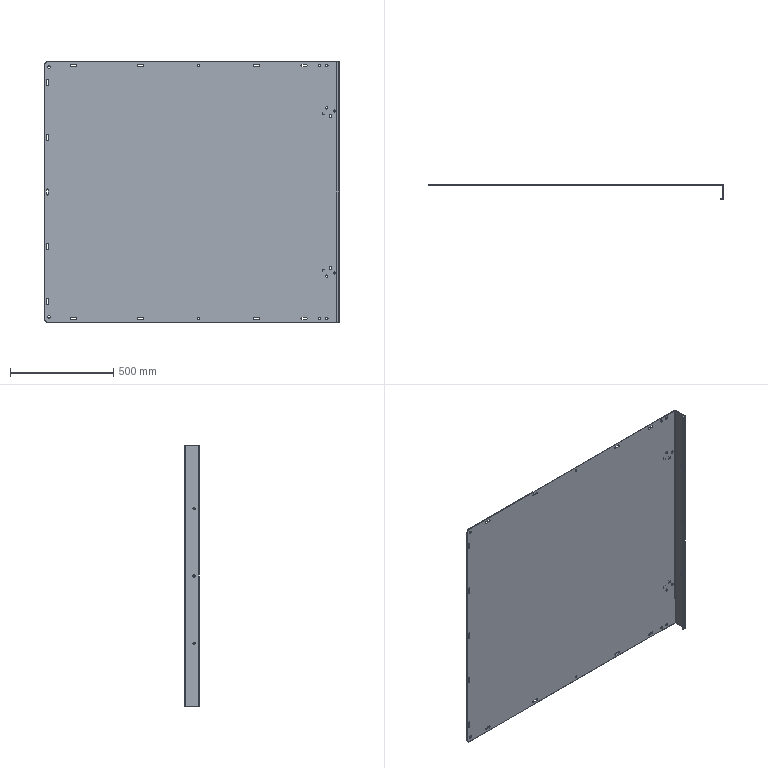Part | SolidWorks | features ICE 10, Cut 1, Fillet 1, FlatPattern 1, SMBaseFlange 1, SheetMetal 1 | 1 solid | 135 faces | box 1425 x 70 x 1260 mm | volume 5663138 mm3 | plane 68 | cylinder 67 | commonest cylinder face diameters 10 x39 10.5 x14 11 x4 12.8 x4 0.4 x2 6.4 x2